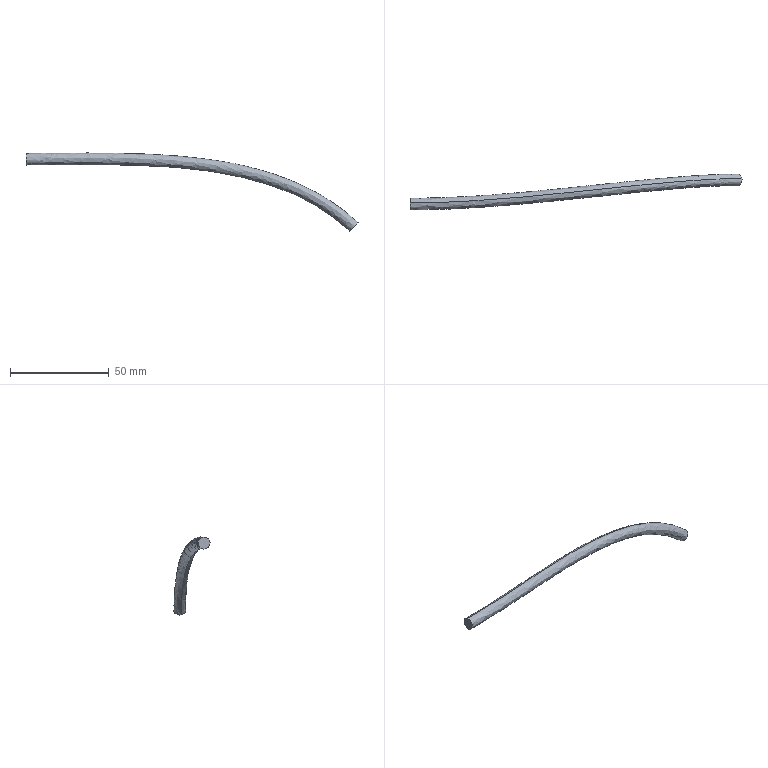Part | SolidWorks | features BaseBody 1 | 1 solid | 4 faces | box 168.028 x 18.28 x 39.544 mm | volume 4926 mm3 | plane 2 | spline 2
STEP:
#1=CARTESIAN_POINT('',(519.168,95.498,6.434));
#2=VERTEX_POINT('',#1);
#3=CARTESIAN_POINT('',(515.186,94.062,2.182));
#4=VERTEX_POINT('',#3);
#5=CARTESIAN_POINT('',(517.177,94.78,4.308));
#6=DIRECTION('',(-0.7299,0.,0.6835));
#7=DIRECTION('',(0.6636,0.2395,0.7087));
#8=AXIS2_PLACEMENT_3D('',#5,#6,#7);
#9=CIRCLE('',#8,3.);
#10=EDGE_CURVE('',#2,#4,#9,.T.);
#11=ORIENTED_EDGE('',*,*,#10,.F.);
#12=CARTESIAN_POINT('',(517.177,94.78,4.308));
#13=DIRECTION('',(-0.7299,0.,0.6835));
#14=DIRECTION('',(-0.6636,-0.2395,-0.7087));
#15=AXIS2_PLACEMENT_3D('',#12,#13,#14);
#16=CIRCLE('',#15,3.);
#17=EDGE_CURVE('',#4,#2,#16,.T.);
#18=ORIENTED_EDGE('',*,*,#17,.F.);
#19=EDGE_LOOP('',(#11,#18));
#20=FACE_OUTER_BOUND('',#19,.T.);
#21=CARTESIAN_POINT('',(517.177,94.78,4.308));
#22=DIRECTION('',(-0.7299,0.,0.6835));
#23=DIRECTION('',(0.,1.,0.));
#24=AXIS2_PLACEMENT_3D('',#21,#22,#23);
#25=PLANE('',#24);
#26=ADVANCED_FACE('',(#20),#25,.F.);
#27=CARTESIAN_POINT('',(351.2,83.066,41.446));
#28=VERTEX_POINT('',#27);
#29=CARTESIAN_POINT('',(519.168,95.498,6.434));
#30=CARTESIAN_POINT('',(514.45,95.498,10.853));
#31=CARTESIAN_POINT('',(503.923,95.175,18.916));
#32=CARTESIAN_POINT('',(486.133,93.894,27.968));
#33=CARTESIAN_POINT('',(465.868,91.952,34.548));
#34=CARTESIAN_POINT('',(436.959,88.882,40.036));
#35=CARTESIAN_POINT('',(397.509,84.79,42.082));
#36=CARTESIAN_POINT('',(366.45,83.066,41.446));
#37=CARTESIAN_POINT('',(351.2,83.066,41.446));
#38=B_SPLINE_CURVE_WITH_KNOTS('',3,(#29,#30,#31,#32,#33,#34,#35,#36,#37),.UNSPECIFIED.,.F.,.F.,(4,1,1,1,1,1,4),(0.,0.1106,0.2304,0.3502,0.48,0.7296,1.),.UNSPECIFIED.);
#39=EDGE_CURVE('',#2,#28,#38,.T.);
#40=ORIENTED_EDGE('',*,*,#39,.T.);
#41=CARTESIAN_POINT('',(351.2,81.934,35.554));
#42=VERTEX_POINT('',#41);
#43=CARTESIAN_POINT('',(351.2,82.5,38.5));
#44=DIRECTION('',(-1.,0.,0.));
#45=DIRECTION('',(0.,-0.1886,-0.982));
#46=AXIS2_PLACEMENT_3D('',#43,#44,#45);
#47=CIRCLE('',#46,3.);
#48=EDGE_CURVE('',#42,#28,#47,.T.);
#49=ORIENTED_EDGE('',*,*,#48,.F.);
#50=CARTESIAN_POINT('',(515.186,94.062,2.182));
#51=CARTESIAN_POINT('',(510.76,94.062,6.327));
#52=CARTESIAN_POINT('',(500.879,93.759,13.899));
#53=CARTESIAN_POINT('',(484.025,92.546,22.488));
#54=CARTESIAN_POINT('',(464.578,90.685,28.811));
#55=CARTESIAN_POINT('',(436.496,87.698,34.153));
#56=CARTESIAN_POINT('',(397.617,83.663,36.189));
#57=CARTESIAN_POINT('',(366.579,81.934,35.554));
#58=CARTESIAN_POINT('',(351.2,81.934,35.554));
#59=B_SPLINE_CURVE_WITH_KNOTS('',3,(#50,#51,#52,#53,#54,#55,#56,#57,#58),.UNSPECIFIED.,.F.,.F.,(4,1,1,1,1,1,4),(0.,0.1106,0.2304,0.3502,0.48,0.7296,1.),.UNSPECIFIED.);
#60=EDGE_CURVE('',#4,#42,#59,.T.);
#61=ORIENTED_EDGE('',*,*,#60,.F.);
#62=ORIENTED_EDGE('',*,*,#17,.T.);
#63=EDGE_LOOP('',(#40,#49,#61,#62));
#64=FACE_OUTER_BOUND('',#63,.T.);
#65=CARTESIAN_POINT('',(516.38,94.242,0.9896));
#66=CARTESIAN_POINT('',(515.976,94.245,1.382));
#67=CARTESIAN_POINT('',(511.172,94.259,5.962));
#68=CARTESIAN_POINT('',(500.852,93.943,13.871));
#69=CARTESIAN_POINT('',(483.998,92.73,22.459));
#70=CARTESIAN_POINT('',(464.551,90.869,28.782));
#71=CARTESIAN_POINT('',(436.473,87.882,34.123));
#72=CARTESIAN_POINT('',(397.601,83.848,36.159));
#73=CARTESIAN_POINT('',(365.971,82.087,35.512));
#74=CARTESIAN_POINT('',(350.057,82.121,35.525));
#75=CARTESIAN_POINT('',(349.487,82.124,35.526));
#76=CARTESIAN_POINT('',(516.603,92.425,1.231));
#77=CARTESIAN_POINT('',(516.199,92.428,1.623));
#78=CARTESIAN_POINT('',(511.402,92.443,6.197));
#79=CARTESIAN_POINT('',(501.093,92.127,14.098));
#80=CARTESIAN_POINT('',(484.246,90.914,22.683));
#81=CARTESIAN_POINT('',(464.795,89.053,29.008));
#82=CARTESIAN_POINT('',(436.694,86.064,34.355));
#83=CARTESIAN_POINT('',(397.76,82.024,36.396));
#84=CARTESIAN_POINT('',(366.038,80.255,35.745));
#85=CARTESIAN_POINT('',(350.052,80.29,35.758));
#86=CARTESIAN_POINT('',(349.479,80.293,35.759));
#87=CARTESIAN_POINT('',(517.679,91.421,2.346));
#88=CARTESIAN_POINT('',(517.27,91.424,2.743));
#89=CARTESIAN_POINT('',(512.406,91.439,7.381));
#90=CARTESIAN_POINT('',(501.953,91.119,15.391));
#91=CARTESIAN_POINT('',(484.901,89.891,24.079));
#92=CARTESIAN_POINT('',(465.263,88.011,30.462));
#93=CARTESIAN_POINT('',(436.959,85.002,35.847));
#94=CARTESIAN_POINT('',(397.852,80.944,37.893));
#95=CARTESIAN_POINT('',(366.057,79.172,37.24));
#96=CARTESIAN_POINT('',(350.05,79.207,37.253));
#97=CARTESIAN_POINT('',(349.477,79.209,37.254));
#98=CARTESIAN_POINT('',(518.929,91.863,3.63));
#99=CARTESIAN_POINT('',(518.512,91.866,4.036));
#100=CARTESIAN_POINT('',(513.55,91.881,8.767));
#101=CARTESIAN_POINT('',(502.889,91.554,16.935));
#102=CARTESIAN_POINT('',(485.549,90.306,25.765));
#103=CARTESIAN_POINT('',(465.66,88.401,32.227));
#104=CARTESIAN_POINT('',(437.102,85.366,37.657));
#105=CARTESIAN_POINT('',(397.818,81.291,39.706));
#106=CARTESIAN_POINT('',(366.017,79.52,39.053));
#107=CARTESIAN_POINT('',(350.053,79.555,39.066));
#108=CARTESIAN_POINT('',(349.482,79.558,39.067));
#109=CARTESIAN_POINT('',(520.179,92.306,4.915));
#110=CARTESIAN_POINT('',(519.753,92.308,5.328));
#111=CARTESIAN_POINT('',(514.694,92.324,10.153));
#112=CARTESIAN_POINT('',(503.826,91.99,18.478));
#113=CARTESIAN_POINT('',(486.198,90.721,27.452));
#114=CARTESIAN_POINT('',(466.057,88.791,33.993));
#115=CARTESIAN_POINT('',(437.244,85.731,39.467));
#116=CARTESIAN_POINT('',(397.785,81.638,41.52));
#117=CARTESIAN_POINT('',(365.978,79.869,40.866));
#118=CARTESIAN_POINT('',(350.056,79.903,40.879));
#119=CARTESIAN_POINT('',(349.486,79.906,40.88));
#120=CARTESIAN_POINT('',(520.814,93.915,5.559));
#121=CARTESIAN_POINT('',(520.383,93.917,5.978));
#122=CARTESIAN_POINT('',(515.257,93.933,10.866));
#123=CARTESIAN_POINT('',(504.248,93.595,19.298));
#124=CARTESIAN_POINT('',(486.431,92.312,28.365));
#125=CARTESIAN_POINT('',(466.133,90.366,34.955));
#126=CARTESIAN_POINT('',(437.174,87.292,40.454));
#127=CARTESIAN_POINT('',(397.648,83.192,42.505));
#128=CARTESIAN_POINT('',(365.904,81.429,41.854));
#129=CARTESIAN_POINT('',(350.062,81.463,41.867));
#130=CARTESIAN_POINT('',(349.495,81.466,41.868));
#131=CARTESIAN_POINT('',(520.434,95.676,5.156));
#132=CARTESIAN_POINT('',(520.004,95.679,5.575));
#133=CARTESIAN_POINT('',(514.883,95.694,10.457));
#134=CARTESIAN_POINT('',(503.889,95.357,18.877));
#135=CARTESIAN_POINT('',(486.102,94.075,27.929));
#136=CARTESIAN_POINT('',(465.84,92.133,34.508));
#137=CARTESIAN_POINT('',(436.935,89.064,39.995));
#138=CARTESIAN_POINT('',(397.493,84.974,42.04));
#139=CARTESIAN_POINT('',(365.842,83.216,41.393));
#140=CARTESIAN_POINT('',(350.067,83.251,41.405));
#141=CARTESIAN_POINT('',(349.502,83.254,41.406));
#142=(BOUNDED_SURFACE()B_SPLINE_SURFACE(3,3,((#65,#66,#67,#68,#69,#70,#71,#72,#73,#74,#75),(#76,#77,#78,#79,#80,#81,#82,#83,#84,#85,#86),(#87,#88,#89,#90,#91,#92,#93,#94,#95,#96,#97),(#98,#99,#100,#101,#102,#103,#104,#105,#106,#107,#108),(#109,#110,#111,#112,#113,#114,#115,#116,#117,#118,#119),(#120,#121,#122,#123,#124,#125,#126,#127,#128,#129,#130),(#131,#132,#133,#134,#135,#136,#137,#138,#139,#140,#141)),.UNSPECIFIED.,.F.,.F.,.T.)B_SPLINE_SURFACE_WITH_KNOTS((4,3,4),(4,1,1,1,1,1,1,1,4),(0.,0.5,1.),(0.,0.01003,0.1184,0.2358,0.3533,0.4805,0.7251,0.9901,1.),.UNSPECIFIED.)GEOMETRIC_REPRESENTATION_ITEM()RATIONAL_B_SPLINE_SURFACE(((1.187,1.187,1.187,1.187,1.187,1.187,1.187,1.187,1.187,1.187,1.187),(0.9376,0.9376,0.9376,0.9376,0.9376,0.9376,0.9376,0.9376,0.9376,0.9376,0.9376),(0.9376,0.9376,0.9376,0.9376,0.9376,0.9376,0.9376,0.9376,0.9376,0.9376,0.9376),(1.187,1.187,1.187,1.187,1.187,1.187,1.187,1.187,1.187,1.187,1.187),(0.9376,0.9376,0.9376,0.9376,0.9376,0.9376,0.9376,0.9376,0.9376,0.9376,0.9376),(0.9376,0.9376,0.9376,0.9376,0.9376,0.9376,0.9376,0.9376,0.9376,0.9376,0.9376),(1.187,1.187,1.187,1.187,1.187,1.187,1.187,1.187,1.187,1.187,1.187)))REPRESENTATION_ITEM('')SURFACE());
#143=ADVANCED_FACE('',(#64),#142,.T.);
#144=ORIENTED_EDGE('',*,*,#60,.T.);
#145=CARTESIAN_POINT('',(351.2,82.5,38.5));
#146=DIRECTION('',(-1.,0.,0.));
#147=DIRECTION('',(0.,0.1886,0.982));
#148=AXIS2_PLACEMENT_3D('',#145,#146,#147);
#149=CIRCLE('',#148,3.);
#150=EDGE_CURVE('',#28,#42,#149,.T.);
#151=ORIENTED_EDGE('',*,*,#150,.F.);
#152=ORIENTED_EDGE('',*,*,#39,.F.);
#153=ORIENTED_EDGE('',*,*,#10,.T.);
#154=EDGE_LOOP('',(#144,#151,#152,#153));
#155=FACE_OUTER_BOUND('',#154,.T.);
#156=CARTESIAN_POINT('',(520.496,95.31,5.222));
#157=CARTESIAN_POINT('',(520.065,95.313,5.641));
#158=CARTESIAN_POINT('',(514.945,95.329,10.523));
#159=CARTESIAN_POINT('',(503.951,94.991,18.944));
#160=CARTESIAN_POINT('',(486.161,93.71,27.997));
#161=CARTESIAN_POINT('',(465.895,91.767,34.577));
#162=CARTESIAN_POINT('',(436.982,88.697,40.065));
#163=CARTESIAN_POINT('',(397.525,84.605,42.112));
#164=CARTESIAN_POINT('',(365.855,82.846,41.464));
#165=CARTESIAN_POINT('',(350.066,82.881,41.476));
#166=CARTESIAN_POINT('',(349.5,82.884,41.477));
#167=CARTESIAN_POINT('',(520.273,97.127,4.981));
#168=CARTESIAN_POINT('',(519.842,97.13,5.4));
#169=CARTESIAN_POINT('',(514.715,97.145,10.288));
#170=CARTESIAN_POINT('',(503.71,96.807,18.717));
#171=CARTESIAN_POINT('',(485.912,95.525,27.773));
#172=CARTESIAN_POINT('',(465.651,93.583,34.351));
#173=CARTESIAN_POINT('',(436.761,90.515,39.833));
#174=CARTESIAN_POINT('',(397.366,86.43,41.875));
#175=CARTESIAN_POINT('',(365.789,84.678,41.23));
#176=CARTESIAN_POINT('',(350.071,84.712,41.243));
#177=CARTESIAN_POINT('',(349.508,84.715,41.244));
#178=CARTESIAN_POINT('',(519.197,98.131,3.866));
#179=CARTESIAN_POINT('',(518.771,98.134,4.28));
#180=CARTESIAN_POINT('',(513.711,98.149,9.104));
#181=CARTESIAN_POINT('',(502.85,97.816,17.424));
#182=CARTESIAN_POINT('',(485.257,96.548,26.377));
#183=CARTESIAN_POINT('',(465.183,94.625,32.897));
#184=CARTESIAN_POINT('',(436.496,91.577,38.342));
#185=CARTESIAN_POINT('',(397.274,87.509,40.378));
#186=CARTESIAN_POINT('',(365.769,85.761,39.735));
#187=CARTESIAN_POINT('',(350.072,85.796,39.748));
#188=CARTESIAN_POINT('',(349.51,85.798,39.749));
#189=CARTESIAN_POINT('',(517.947,97.689,2.581));
#190=CARTESIAN_POINT('',(517.529,97.691,2.987));
#191=CARTESIAN_POINT('',(512.567,97.707,7.718));
#192=CARTESIAN_POINT('',(501.913,97.38,15.88));
#193=CARTESIAN_POINT('',(484.609,96.134,24.691));
#194=CARTESIAN_POINT('',(464.786,94.235,31.132));
#195=CARTESIAN_POINT('',(436.353,91.213,36.532));
#196=CARTESIAN_POINT('',(397.307,87.162,38.565));
#197=CARTESIAN_POINT('',(365.809,85.413,37.922));
#198=CARTESIAN_POINT('',(350.069,85.447,37.935));
#199=CARTESIAN_POINT('',(349.506,85.45,37.936));
#200=CARTESIAN_POINT('',(516.697,97.247,1.297));
#201=CARTESIAN_POINT('',(516.288,97.249,1.694));
#202=CARTESIAN_POINT('',(511.423,97.264,6.332));
#203=CARTESIAN_POINT('',(500.977,96.944,14.337));
#204=CARTESIAN_POINT('',(483.96,95.719,23.004));
#205=CARTESIAN_POINT('',(464.389,93.845,29.366));
#206=CARTESIAN_POINT('',(436.211,90.849,34.721));
#207=CARTESIAN_POINT('',(397.341,86.815,36.752));
#208=CARTESIAN_POINT('',(365.849,85.065,36.109));
#209=CARTESIAN_POINT('',(350.066,85.099,36.122));
#210=CARTESIAN_POINT('',(349.501,85.102,36.122));
#211=CARTESIAN_POINT('',(516.061,95.637,0.6527));
#212=CARTESIAN_POINT('',(515.658,95.64,1.045));
#213=CARTESIAN_POINT('',(510.86,95.655,5.619));
#214=CARTESIAN_POINT('',(500.554,95.339,13.517));
#215=CARTESIAN_POINT('',(483.727,94.128,22.091));
#216=CARTESIAN_POINT('',(464.313,92.27,28.404));
#217=CARTESIAN_POINT('',(436.281,89.288,33.735));
#218=CARTESIAN_POINT('',(397.478,85.261,35.766));
#219=CARTESIAN_POINT('',(365.923,83.504,35.122));
#220=CARTESIAN_POINT('',(350.061,83.539,35.134));
#221=CARTESIAN_POINT('',(349.492,83.542,35.135));
#222=CARTESIAN_POINT('',(516.442,93.876,1.055));
#223=CARTESIAN_POINT('',(516.037,93.879,1.448));
#224=CARTESIAN_POINT('',(511.234,93.893,6.028));
#225=CARTESIAN_POINT('',(500.913,93.578,13.937));
#226=CARTESIAN_POINT('',(484.057,92.364,22.527));
#227=CARTESIAN_POINT('',(464.606,90.503,28.851));
#228=CARTESIAN_POINT('',(436.52,87.515,34.194));
#229=CARTESIAN_POINT('',(397.633,83.48,36.231));
#230=CARTESIAN_POINT('',(365.984,81.717,35.583));
#231=CARTESIAN_POINT('',(350.056,81.751,35.596));
#232=CARTESIAN_POINT('',(349.485,81.754,35.597));
#233=(BOUNDED_SURFACE()B_SPLINE_SURFACE(3,3,((#156,#157,#158,#159,#160,#161,#162,#163,#164,#165,#166),(#167,#168,#169,#170,#171,#172,#173,#174,#175,#176,#177),(#178,#179,#180,#181,#182,#183,#184,#185,#186,#187,#188),(#189,#190,#191,#192,#193,#194,#195,#196,#197,#198,#199),(#200,#201,#202,#203,#204,#205,#206,#207,#208,#209,#210),(#211,#212,#213,#214,#215,#216,#217,#218,#219,#220,#221),(#222,#223,#224,#225,#226,#227,#228,#229,#230,#231,#232)),.UNSPECIFIED.,.F.,.F.,.T.)B_SPLINE_SURFACE_WITH_KNOTS((4,3,4),(4,1,1,1,1,1,1,1,4),(0.,0.5,1.),(0.,0.01003,0.1184,0.2358,0.3533,0.4805,0.7251,0.9901,1.),.UNSPECIFIED.)GEOMETRIC_REPRESENTATION_ITEM()RATIONAL_B_SPLINE_SURFACE(((1.187,1.187,1.187,1.187,1.187,1.187,1.187,1.187,1.187,1.187,1.187),(0.9376,0.9376,0.9376,0.9376,0.9376,0.9376,0.9376,0.9376,0.9376,0.9376,0.9376),(0.9376,0.9376,0.9376,0.9376,0.9376,0.9376,0.9376,0.9376,0.9376,0.9376,0.9376),(1.187,1.187,1.187,1.187,1.187,1.187,1.187,1.187,1.187,1.187,1.187),(0.9376,0.9376,0.9376,0.9376,0.9376,0.9376,0.9376,0.9376,0.9376,0.9376,0.9376),(0.9376,0.9376,0.9376,0.9376,0.9376,0.9376,0.9376,0.9376,0.9376,0.9376,0.9376),(1.187,1.187,1.187,1.187,1.187,1.187,1.187,1.187,1.187,1.187,1.187)))REPRESENTATION_ITEM('')SURFACE());
#234=ADVANCED_FACE('',(#155),#233,.T.);
#235=ORIENTED_EDGE('',*,*,#150,.T.);
#236=ORIENTED_EDGE('',*,*,#48,.T.);
#237=EDGE_LOOP('',(#235,#236));
#238=FACE_OUTER_BOUND('',#237,.T.);
#239=CARTESIAN_POINT('',(351.2,82.5,38.5));
#240=DIRECTION('',(-1.,0.,0.));
#241=DIRECTION('',(0.,0.,1.));
#242=AXIS2_PLACEMENT_3D('',#239,#240,#241);
#243=PLANE('',#242);
#244=ADVANCED_FACE('',(#238),#243,.T.);
#245=CLOSED_SHELL('',(#26,#143,#234,#244));
#246=MANIFOLD_SOLID_BREP('',#245);
#247=CARTESIAN_POINT('',(0.,0.,0.));
#248=DIRECTION('',(0.,0.,1.));
#249=DIRECTION('',(1.,0.,0.));
#250=AXIS2_PLACEMENT_3D('',#247,#248,#249);
#251=(LENGTH_UNIT()NAMED_UNIT(*)SI_UNIT(.MILLI.,.METRE.));
#252=UNCERTAINTY_MEASURE_WITH_UNIT(LENGTH_MEASURE(0.00001),#251,'','');
#253=(NAMED_UNIT(*)PLANE_ANGLE_UNIT()SI_UNIT($,.RADIAN.));
#254=(NAMED_UNIT(*)SI_UNIT($,.STERADIAN.)SOLID_ANGLE_UNIT());
#255=(GEOMETRIC_REPRESENTATION_CONTEXT(3)GLOBAL_UNCERTAINTY_ASSIGNED_CONTEXT((#252))GLOBAL_UNIT_ASSIGNED_CONTEXT((#251,#253,#254))REPRESENTATION_CONTEXT('',''));
#256=ADVANCED_BREP_SHAPE_REPRESENTATION('',(#246,#250),#255);